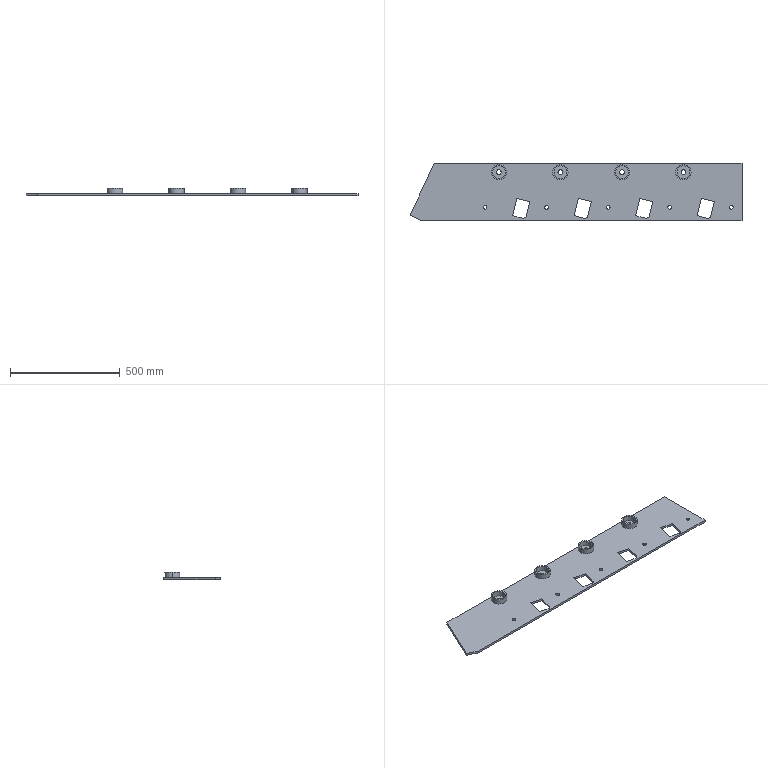Part | STEP file | Edge plate 7_Default<As machined> | 5 solids | 69 faces | box 1511 x 260 x 35 mm | volume 3690417 mm3 | cylinder 38 | plane 31 | commonest cylinder face diameters 17 x10 22 x8 58 x8 70 x8 30 x4